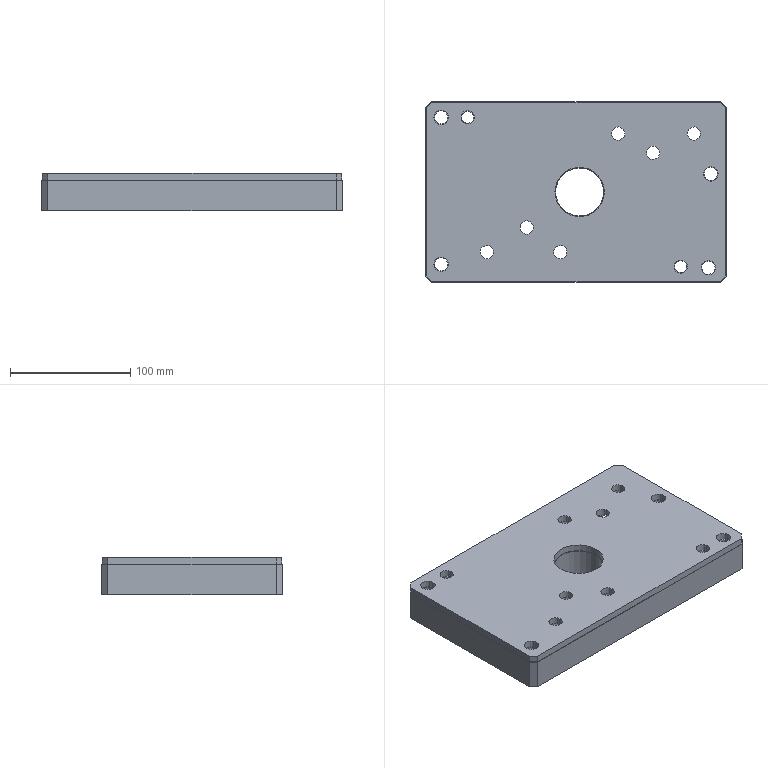Part | CATIA | 2 solids | 121 faces | box 250 x 150 x 30.8 mm | volume 950140 mm3 | cylinder 73 | plane 36 | other 12 | commonest cylinder face diameters 11 x24 10 x8 12 x8 18 x8 40 x6 6 x4